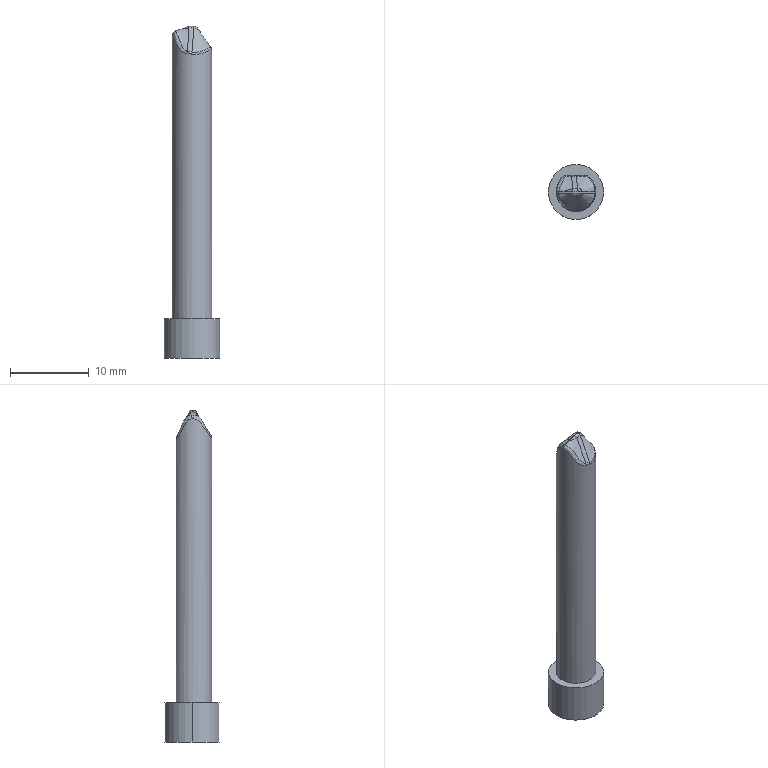Part | 1 solid | 32 faces | box 7 x 7 x 42.035 mm | volume 850.375 mm3 | spline 18 | cylinder 6 | plane 5 | other 3 | commonest cylinder face diameters 0.7 x2 7 x2 1.4 x1 5 x1